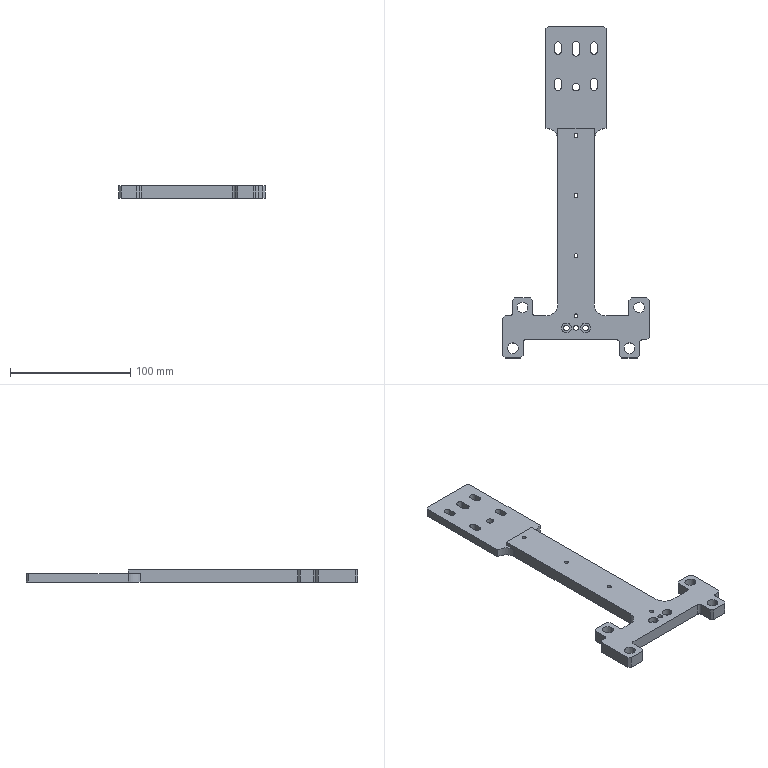Part | STEP file | 10-19 suction plate fixing block | 1 solid | 98 faces | box 122 x 276 x 10 mm | volume 105973 mm3 | plane 50 | cylinder 48 | commonest cylinder face diameters 3.3 x8 4 x8 5.5 x8 9 x8 4.5 x4 6 x4